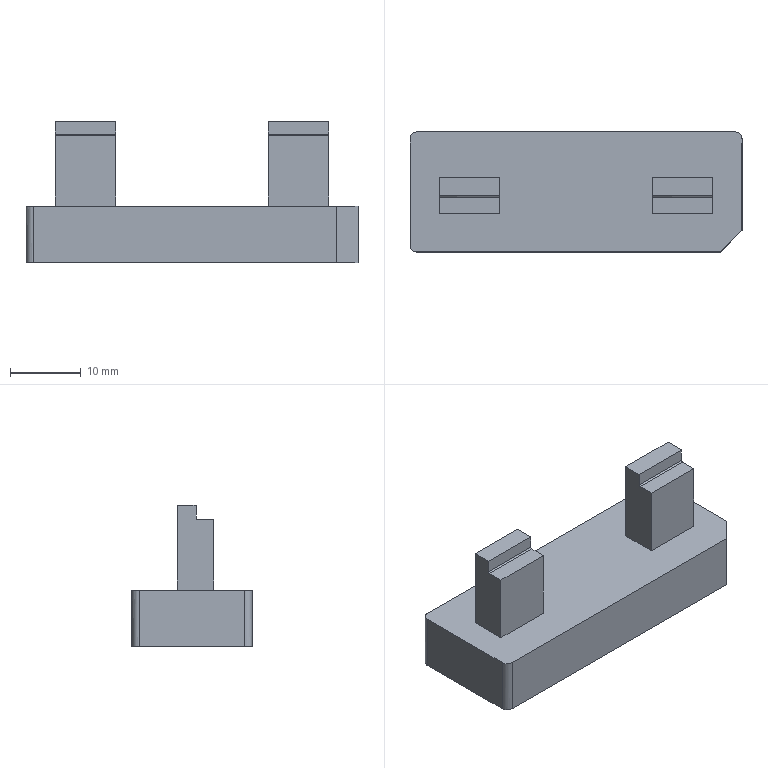NC program | PowerMill | posted by the shop | part box 47 x 17 x 19.985 mm
Lines 5811 to 7380 of 62704:
( TOOL ID   D4C_1_1 )
( TOOL DIA. 4. TIP RAD 0 LENGTH 67.16 )
( Z = -12.11 )
T2 M6
T3
G91 G28 Z0
G0 G90 G54
M08
S18000 M3
X0 Y0 M8
G43 Z9.805 H2
X-13.691 Y-3.55
Z.799
G1 Z-.401 F3600
X-13.681 Y-3.53 F6000
G3 X-13.77 Y-3.264 I-.177 J.089
G1 X-15.13 Y-2.584
X-19.278
X-19.766 Y-2.535
X-20.254 Y-2.355
X-20.509 Y-2.196
X-20.742 Y-1.995
X-20.979 Y-1.708
X-21.221 Y-1.22
X-21.319 Y-.732
X-21.322 Y2.196
X-21.23 Y2.701
X-21.008 Y3.172
X-20.742 Y3.504
X-20.567 Y3.66
X-20.254 Y3.864
X-19.766 Y4.043
X-19.278 Y4.093
X-10.981
X-10.493 Y4.065
X-10.005 Y3.917
X-9.583 Y3.66
X-9.141 Y3.172
X-9.029 Y2.973
X-8.915 Y2.684
X-8.828 Y2.196
X-8.831 Y-.732
X-8.929 Y-1.22
X-9.029 Y-1.464
X-9.171 Y-1.708
X-9.517 Y-2.097
X-9.641 Y-2.196
X-10.005 Y-2.408
X-10.493 Y-2.557
X-10.981 Y-2.584
X-15.13
X-13.691 Y-3.55 Z-.597
X-13.681 Y-3.53
G3 X-13.77 Y-3.264 I-.177 J.089
G1 X-15.13 Y-2.584
X-19.278
X-19.766 Y-2.535
X-20.254 Y-2.355
X-20.509 Y-2.196
X-20.742 Y-1.995
X-20.979 Y-1.708
X-21.221 Y-1.22
X-21.319 Y-.732
X-21.322 Y2.196
X-21.23 Y2.701
X-21.008 Y3.172
X-20.742 Y3.504
X-20.567 Y3.66
X-20.254 Y3.864
X-19.766 Y4.043
X-19.278 Y4.093
X-10.981
X-10.493 Y4.065
X-10.005 Y3.917
X-9.583 Y3.66
X-9.141 Y3.172
X-9.029 Y2.973
X-8.915 Y2.684
X-8.828 Y2.196
X-8.83 Y-.732
X-8.929 Y-1.22
X-9.029 Y-1.464
X-9.171 Y-1.708
X-9.517 Y-2.097
X-9.641 Y-2.196
X-10.005 Y-2.408
X-10.493 Y-2.557
X-10.981 Y-2.584
X-15.13
X-13.691 Y-3.55 Z-.793
X-13.681 Y-3.53
G3 X-13.77 Y-3.264 I-.177 J.089
G1 X-15.13 Y-2.584
X-19.278
X-19.766 Y-2.535
X-20.254 Y-2.355
X-20.509 Y-2.196
X-20.742 Y-1.995
X-20.979 Y-1.708
X-21.221 Y-1.22
X-21.319 Y-.732
X-21.322 Y2.196
X-21.23 Y2.701
X-21.008 Y3.172
X-20.742 Y3.504
X-20.567 Y3.66
X-20.254 Y3.864
X-19.766 Y4.043
X-19.278 Y4.093
X-10.981
X-10.493 Y4.065
X-10.005 Y3.917
X-9.583 Y3.66
X-9.141 Y3.172
X-9.029 Y2.973
X-8.915 Y2.684
X-8.828 Y2.196
X-8.83 Y-.732
X-8.929 Y-1.22
X-9.029 Y-1.464
X-9.171 Y-1.708
X-9.517 Y-2.097
X-9.641 Y-2.196
X-10.005 Y-2.409
X-10.493 Y-2.557
X-10.981 Y-2.584
X-15.13
X-13.691 Y-3.55 Z-.989
X-13.681 Y-3.53
G3 X-13.77 Y-3.264 I-.177 J.089
G1 X-15.13 Y-2.584
X-19.278
X-19.766 Y-2.535
X-20.254 Y-2.355
X-20.509 Y-2.196
X-20.742 Y-1.995
X-20.979 Y-1.708
X-21.221 Y-1.22
X-21.319 Y-.732
X-21.322 Y2.196
X-21.23 Y2.701
X-21.008 Y3.172
X-20.742 Y3.504
X-20.567 Y3.66
X-20.254 Y3.864
X-19.766 Y4.043
X-19.278 Y4.093
X-10.981
X-10.493 Y4.065
X-10.005 Y3.917
X-9.583 Y3.66
X-9.141 Y3.172
X-9.029 Y2.973
X-8.915 Y2.684
X-8.828 Y2.196
X-8.83 Y-.732
X-8.929 Y-1.22
X-9.029 Y-1.464
X-9.171 Y-1.708
X-9.517 Y-2.097
X-9.641 Y-2.196
X-10.005 Y-2.409
X-10.493 Y-2.557
X-10.981 Y-2.584
X-15.13
X-13.691 Y-3.55 Z-1.185
X-13.681 Y-3.53
G3 X-13.77 Y-3.264 I-.177 J.089
G1 X-15.13 Y-2.584
X-19.278
X-19.766 Y-2.535
X-20.254 Y-2.355
X-20.509 Y-2.196
X-20.742 Y-1.996
X-20.979 Y-1.708
X-21.221 Y-1.22
X-21.32 Y-.732
X-21.322 Y2.196
X-21.23 Y2.701
X-21.008 Y3.172
X-20.742 Y3.504
X-20.567 Y3.66
X-20.254 Y3.864
X-19.766 Y4.043
X-19.278 Y4.093
X-10.981
X-10.493 Y4.065
X-10.005 Y3.917
X-9.583 Y3.66
X-9.141 Y3.172
X-9.029 Y2.973
X-8.915 Y2.684
X-8.828 Y2.196
X-8.83 Y-.732
X-8.929 Y-1.22
X-9.029 Y-1.464
X-9.171 Y-1.708
X-9.517 Y-2.097
X-9.641 Y-2.196
X-10.005 Y-2.409
X-10.493 Y-2.557
X-10.981 Y-2.584
X-15.13
X-13.691 Y-3.55 Z-1.381
X-13.681 Y-3.53
G3 X-13.77 Y-3.264 I-.177 J.089
G1 X-15.13 Y-2.584
X-19.278
X-19.766 Y-2.535
X-20.254 Y-2.355
X-20.509 Y-2.196
X-20.742 Y-1.996
X-20.979 Y-1.708
X-21.221 Y-1.22
X-21.32 Y-.732
X-21.322 Y2.196
X-21.23 Y2.701
X-21.008 Y3.172
X-20.742 Y3.504
X-20.567 Y3.66
X-20.254 Y3.864
X-19.766 Y4.043
X-19.278 Y4.093
X-10.981
X-10.493 Y4.065
X-10.005 Y3.917
X-9.583 Y3.66
X-9.141 Y3.172
X-9.029 Y2.973
X-8.915 Y2.684
X-8.828 Y2.196
X-8.83 Y-.732
X-8.929 Y-1.22
X-9.029 Y-1.464
X-9.171 Y-1.708
X-9.517 Y-2.097
X-9.641 Y-2.196
X-10.005 Y-2.409
X-10.493 Y-2.557
X-10.981 Y-2.584
X-15.13
X-13.691 Y-3.55 Z-1.577
X-13.681 Y-3.53
G3 X-13.77 Y-3.264 I-.177 J.089
G1 X-15.13 Y-2.584
X-19.278
X-19.766 Y-2.535
X-20.254 Y-2.355
X-20.509 Y-2.196
X-20.742 Y-1.996
X-20.979 Y-1.708
X-21.221 Y-1.22
X-21.32 Y-.732
X-21.322 Y2.196
X-21.23 Y2.701
X-21.008 Y3.172
X-20.742 Y3.504
X-20.567 Y3.66
X-20.254 Y3.864
X-19.766 Y4.043
X-19.278 Y4.093
X-10.981
X-10.493 Y4.065
X-10.005 Y3.917
X-9.583 Y3.66
X-9.141 Y3.172
X-9.029 Y2.973
X-8.915 Y2.684
X-8.828 Y2.196
X-8.83 Y-.732
X-8.929 Y-1.22
X-9.029 Y-1.464
X-9.171 Y-1.708
X-9.517 Y-2.097
X-9.641 Y-2.196
X-10.005 Y-2.409
X-10.493 Y-2.557
X-10.981 Y-2.584
X-15.13
X-13.691 Y-3.55 Z-1.773
X-13.681 Y-3.53
G3 X-13.77 Y-3.264 I-.177 J.089
G1 X-15.13 Y-2.584
X-19.278
X-19.766 Y-2.535
X-20.254 Y-2.355
X-20.509 Y-2.196
X-20.742 Y-1.996
X-20.979 Y-1.708
X-21.221 Y-1.22
X-21.32 Y-.732
X-21.322 Y2.196
X-21.23 Y2.701
X-21.008 Y3.172
X-20.742 Y3.504
X-20.567 Y3.66
X-20.254 Y3.864
X-19.766 Y4.043
X-19.278 Y4.093
X-10.981
X-10.493 Y4.065
X-10.005 Y3.917
X-9.583 Y3.66
X-9.141 Y3.172
X-9.029 Y2.973
X-8.915 Y2.684
X-8.828 Y2.196
X-8.83 Y-.732
X-8.929 Y-1.22
X-9.029 Y-1.464
X-9.171 Y-1.708
X-9.517 Y-2.097
X-9.641 Y-2.196
X-10.005 Y-2.409
X-10.493 Y-2.557
X-10.981 Y-2.584
X-15.13
X-13.608 Y-3.591 Z-1.969
X-13.598 Y-3.571
G3 X-13.687 Y-3.306 I-.177 J.089
G1 X-15.13 Y-2.584
X-19.278
X-19.766 Y-2.535
X-20.254 Y-2.355
X-20.509 Y-2.196
X-20.742 Y-1.996
X-20.979 Y-1.708
X-21.221 Y-1.22
X-21.32 Y-.732
X-21.322 Y2.196
X-21.23 Y2.701
X-21.008 Y3.172
X-20.742 Y3.504
X-20.567 Y3.66
X-20.254 Y3.864
X-19.766 Y4.043
X-19.278 Y4.093
X-10.981
X-10.493 Y4.065
X-10.005 Y3.917
X-9.583 Y3.66
X-9.141 Y3.172
X-9.029 Y2.973
X-8.915 Y2.684
X-8.828 Y2.196
X-8.83 Y-.732
X-8.929 Y-1.22
X-9.029 Y-1.464
X-9.171 Y-1.708
X-9.517 Y-2.097
X-9.641 Y-2.196
X-10.005 Y-2.409
X-10.493 Y-2.557
X-10.981 Y-2.584
X-15.13
X-13.704 Y-3.64 Z-2.165
X-13.695 Y-3.62
G3 X-13.783 Y-3.354 I-.177 J.089
G1 X-15.13 Y-2.681
X-18.302
X-19.278 Y-2.686
X-19.766 Y-2.639
X-20.254 Y-2.458
X-20.636 Y-2.196
X-20.742 Y-2.097
X-21.046 Y-1.708
X-21.23 Y-1.294
X-21.324 Y-.732
X-21.322 Y2.196
X-21.23 Y2.701
X-21.008 Y3.172
X-20.742 Y3.504
X-20.567 Y3.66
X-20.254 Y3.864
X-19.766 Y4.043
X-19.278 Y4.093
X-10.981
X-10.493 Y4.065
X-10.005 Y3.917
X-9.583 Y3.66
X-9.141 Y3.172
X-9.029 Y2.973
X-8.915 Y2.684
X-8.828 Y2.196
X-8.826 Y-.732
X-8.899 Y-1.22
X-9.107 Y-1.708
X-9.517 Y-2.2
X-10.005 Y-2.506
X-10.493 Y-2.655
X-10.981 Y-2.681
X-15.13
G0 Z2.864
G1 X-13.691 Y-6.057 F10000
G0 Z-1.164
G1 Z-2.364 F3600
X-13.681 Y-6.038 F6000
G3 X-13.77 Y-5.772 I-.177 J.089
G1 X-15.13 Y-5.092
X-19.278
X-19.766 Y-5.043
X-20.254 Y-4.863
X-20.596 Y-4.637
X-20.742 Y-4.503
X-21.023 Y-4.148
X-21.23 Y-3.7
X-21.323 Y-3.172
Y-.757
Y-.745
X-21.324 Y-.732
X-21.322 Y2.105
Y2.196
X-21.23 Y2.701
X-21.008 Y3.172
X-20.742 Y3.504
X-20.567 Y3.66
X-20.254 Y3.864
X-19.766 Y4.043
X-19.278 Y4.093
X-10.981
X-10.493 Y4.065
X-10.005 Y3.917
X-9.583 Y3.66
X-9.141 Y3.172
X-9.029 Y2.973
X-8.915 Y2.684
X-8.828 Y2.196
Y2.103
X-8.826 Y-.732
X-8.827 Y-.742
Y-3.172
X-8.907 Y-3.66
X-9.029 Y-3.972
X-9.127 Y-4.148
X-9.554 Y-4.637
X-10.005 Y-4.916
X-10.493 Y-5.064
X-10.981 Y-5.092
X-15.13
X-13.691 Y-6.057 Z-2.563
X-13.681 Y-6.038
G3 X-13.77 Y-5.772 I-.177 J.089
G1 X-15.13 Y-5.092
X-19.278
X-19.766 Y-5.043
X-20.254 Y-4.863
X-20.596 Y-4.637
X-20.742 Y-4.503
X-21.023 Y-4.148
X-21.23 Y-3.7
X-21.323 Y-3.172
Y-.757
Y-.744
X-21.324 Y-.732
X-21.322 Y2.013
Y2.196
X-21.23 Y2.701
X-21.008 Y3.172
X-20.742 Y3.504
X-20.567 Y3.66
X-20.254 Y3.864
X-19.766 Y4.043
X-19.278 Y4.093
X-10.981
X-10.493 Y4.065
X-10.005 Y3.917
X-9.583 Y3.66
X-9.141 Y3.172
X-9.029 Y2.973
X-8.915 Y2.684
X-8.828 Y2.196
Y2.008
X-8.826 Y-.732
X-8.827 Y-.742
Y-3.172
X-8.907 Y-3.66
X-9.029 Y-3.972
X-9.127 Y-4.148
X-9.554 Y-4.637
X-10.005 Y-4.916
X-10.493 Y-5.064
X-10.981 Y-5.092
X-15.13
X-13.691 Y-6.057 Z-2.762
X-13.681 Y-6.038
G3 X-13.77 Y-5.772 I-.177 J.089
G1 X-15.13 Y-5.092
X-19.278
X-19.766 Y-5.043
X-20.254 Y-4.863
X-20.596 Y-4.637
X-20.742 Y-4.503
X-21.023 Y-4.148
X-21.23 Y-3.7
X-21.323 Y-3.172
Y-.756
Y-.744
X-21.324 Y-.732
X-21.322 Y1.922
Y2.196
X-21.23 Y2.701
X-21.009 Y3.172
X-20.742 Y3.504
X-20.567 Y3.66
X-20.254 Y3.864
X-19.766 Y4.043
X-19.278 Y4.093
X-10.981
X-10.493 Y4.065
X-10.005 Y3.917
X-9.583 Y3.66
X-9.141 Y3.172
X-9.029 Y2.973
X-8.915 Y2.684
X-8.828 Y2.196
Y1.913
X-8.826 Y-.732
X-8.827 Y-.742
Y-3.172
X-8.907 Y-3.66
X-9.029 Y-3.972
X-9.127 Y-4.148
X-9.554 Y-4.637
X-10.005 Y-4.916
X-10.493 Y-5.064
X-10.981 Y-5.092
X-15.13
X-13.691 Y-6.057 Z-2.961
X-13.681 Y-6.038
G3 X-13.77 Y-5.772 I-.177 J.089
G1 X-15.13 Y-5.092
X-19.278
X-19.766 Y-5.043
X-20.254 Y-4.863
X-20.596 Y-4.637
X-20.742 Y-4.503
X-21.023 Y-4.148
X-21.23 Y-3.7
X-21.323 Y-3.172
Y-.756
Y-.744
X-21.324 Y-.732
X-21.322 Y1.83
Y2.196
X-21.23 Y2.701
X-21.009 Y3.172
X-20.742 Y3.504
X-20.567 Y3.66
X-20.254 Y3.864
X-19.766 Y4.043
X-19.278 Y4.093
X-10.981
X-10.493 Y4.065
X-10.005 Y3.917
X-9.583 Y3.66
X-9.141 Y3.172
X-9.029 Y2.973
X-8.915 Y2.684
X-8.828 Y2.196
Y1.818
X-8.826 Y-.732
X-8.827 Y-.741
Y-3.172
X-8.907 Y-3.66
X-9.029 Y-3.972
X-9.127 Y-4.148
X-9.554 Y-4.637
X-10.005 Y-4.916
X-10.493 Y-5.064
X-10.981 Y-5.092
X-15.13
X-13.691 Y-6.057 Z-3.16
X-13.681 Y-6.038
G3 X-13.77 Y-5.772 I-.177 J.089
G1 X-15.13 Y-5.092
X-19.278
X-19.766 Y-5.043
X-20.254 Y-4.863
X-20.596 Y-4.637
X-20.742 Y-4.503
X-21.023 Y-4.148
X-21.23 Y-3.7
X-21.323 Y-3.172
Y-.756
Y-.744
X-21.324 Y-.732
X-21.322 Y1.738
Y2.196
X-21.23 Y2.701
X-21.009 Y3.172
X-20.742 Y3.504
X-20.567 Y3.66
X-20.254 Y3.864
X-19.766 Y4.043
X-19.278 Y4.093
X-10.981
X-10.493 Y4.065
X-10.005 Y3.917
X-9.583 Y3.66
X-9.141 Y3.172
X-9.029 Y2.973
X-8.915 Y2.684
X-8.828 Y2.196
Y1.723
X-8.826 Y-.732
X-8.827 Y-.741
Y-3.172
X-8.907 Y-3.66
X-9.029 Y-3.972
X-9.127 Y-4.148
X-9.554 Y-4.637
X-10.005 Y-4.916
X-10.493 Y-5.064
X-10.981 Y-5.092
X-15.13
X-13.691 Y-6.057 Z-3.358
X-13.681 Y-6.038
G3 X-13.77 Y-5.772 I-.177 J.089
G1 X-15.13 Y-5.092
X-19.278
X-19.766 Y-5.043
X-20.254 Y-4.863
X-20.596 Y-4.637
X-20.742 Y-4.503
X-21.023 Y-4.148
X-21.23 Y-3.7
X-21.323 Y-3.172
Y-.755
Y-.744
X-21.324 Y-.732
X-21.322 Y1.647
Y2.196
X-21.23 Y2.701
X-21.009 Y3.172
X-20.742 Y3.504
X-20.567 Y3.66
X-20.254 Y3.864
X-19.766 Y4.043
X-19.278 Y4.093
X-10.981
X-10.493 Y4.065
X-10.005 Y3.917
X-9.583 Y3.66
X-9.141 Y3.172
X-9.029 Y2.973
X-8.915 Y2.684
X-8.828 Y2.196
Y1.628
X-8.826 Y-.732
X-8.827 Y-.741
Y-3.172
X-8.907 Y-3.66
X-9.029 Y-3.972
X-9.127 Y-4.148
X-9.554 Y-4.637
X-10.005 Y-4.916
X-10.493 Y-5.064
X-10.981 Y-5.092
X-15.13
X-13.691 Y-6.057 Z-3.557
X-13.681 Y-6.038
G3 X-13.77 Y-5.772 I-.177 J.089
G1 X-15.13 Y-5.092
X-19.278
X-19.766 Y-5.043
X-20.254 Y-4.863
X-20.596 Y-4.637
X-20.742 Y-4.503
X-21.023 Y-4.148
X-21.23 Y-3.7
X-21.323 Y-3.172
Y-.755
Y-.743
X-21.324 Y-.732
X-21.322 Y1.555
Y2.196
X-21.23 Y2.701
X-21.009 Y3.172
X-20.742 Y3.504
X-20.567 Y3.66
X-20.254 Y3.864
X-19.766 Y4.043
X-19.278 Y4.093
X-10.981
X-10.493 Y4.065
X-10.005 Y3.917
X-9.583 Y3.66
X-9.141 Y3.172
X-9.029 Y2.973
X-8.914 Y2.684
X-8.828 Y2.196
Y1.533
X-8.826 Y-.732
X-8.827 Y-.74
Y-3.172
X-8.907 Y-3.66
X-9.029 Y-3.972
X-9.127 Y-4.148
X-9.554 Y-4.637
X-10.005 Y-4.916
X-10.493 Y-5.064
X-10.981 Y-5.092
X-15.13
X-13.691 Y-6.057 Z-3.756
X-13.681 Y-6.038
G3 X-13.77 Y-5.772 I-.177 J.089
G1 X-15.13 Y-5.092
X-19.278
X-19.766 Y-5.043
X-20.254 Y-4.863
X-20.596 Y-4.637
X-20.742 Y-4.503
X-21.023 Y-4.148
X-21.23 Y-3.7
X-21.323 Y-3.172
Y-.754
Y-.743
X-21.324 Y-.732
X-21.322 Y1.464
Y2.196
X-21.23 Y2.701
X-21.009 Y3.172
X-20.742 Y3.504
X-20.567 Y3.66
X-20.254 Y3.864
X-19.766 Y4.043
X-19.278 Y4.093
X-10.981
X-10.493 Y4.065
X-10.005 Y3.917
X-9.583 Y3.66
X-9.141 Y3.172
X-9.029 Y2.973
X-8.914 Y2.684
X-8.828 Y2.196
Y1.438
X-8.826 Y-.732
X-8.827 Y-.74
Y-3.172
X-8.907 Y-3.66
X-9.029 Y-3.972
X-9.127 Y-4.148
X-9.554 Y-4.637
X-10.005 Y-4.916
X-10.493 Y-5.064
X-10.981 Y-5.092
X-15.13
X-13.691 Y-6.057 Z-3.955
X-13.681 Y-6.038
G3 X-13.77 Y-5.772 I-.177 J.089
G1 X-15.13 Y-5.092
X-19.278
X-19.766 Y-5.043
X-20.254 Y-4.863
X-20.596 Y-4.637
X-20.742 Y-4.503
X-21.023 Y-4.148
X-21.23 Y-3.7
X-21.323 Y-3.172
Y-.754
Y-.743
X-21.324 Y-.732
X-21.322 Y1.372
Y2.196
X-21.23 Y2.701
X-21.009 Y3.172
X-20.742 Y3.504
X-20.567 Y3.66
X-20.254 Y3.864
X-19.766 Y4.043
X-19.278 Y4.093
X-10.981
X-10.493 Y4.065
X-10.005 Y3.917
X-9.583 Y3.66
X-9.141 Y3.172
X-9.029 Y2.973
X-8.914 Y2.684
X-8.828 Y2.196
Y1.344
X-8.826 Y-.732
X-8.827 Y-.74
Y-3.172
X-8.907 Y-3.66
X-9.029 Y-3.972
X-9.127 Y-4.148
X-9.554 Y-4.637
X-10.005 Y-4.916
X-10.493 Y-5.064
X-10.981 Y-5.092
X-15.13
X-13.691 Y-6.057 Z-4.154
X-13.681 Y-6.038
G3 X-13.77 Y-5.772 I-.177 J.089
G1 X-15.13 Y-5.092
X-19.278
X-19.766 Y-5.043
X-20.254 Y-4.863
X-20.596 Y-4.637
X-20.742 Y-4.503
X-21.023 Y-4.148
X-21.23 Y-3.7
X-21.323 Y-3.172
Y-.753
Y-.743
X-21.324 Y-.732
X-21.322 Y1.28
Y2.196
X-21.23 Y2.701
X-21.009 Y3.172
X-20.742 Y3.504
X-20.567 Y3.66
X-20.254 Y3.864
X-19.766 Y4.043
X-19.278 Y4.093
X-10.981
X-10.493 Y4.065
X-10.005 Y3.917
X-9.583 Y3.66
X-9.141 Y3.172
X-9.029 Y2.973
X-8.914 Y2.684
X-8.828 Y2.196
X-8.827 Y1.249
X-8.826 Y-.732
X-8.827 Y-.739
Y-3.172
X-8.907 Y-3.66
X-9.029 Y-3.972
X-9.127 Y-4.148
X-9.554 Y-4.637
X-10.005 Y-4.916
X-10.493 Y-5.064
X-10.981 Y-5.092
X-15.13
X-13.691 Y-6.057 Z-4.353
X-13.681 Y-6.038
G3 X-13.77 Y-5.772 I-.177 J.089
G1 X-15.13 Y-5.092
X-19.278
X-19.766 Y-5.043
X-20.254 Y-4.863
X-20.596 Y-4.637
X-20.742 Y-4.503
X-21.023 Y-4.148
X-21.23 Y-3.7
X-21.323 Y-3.172
Y-.753
Y-.742
X-21.324 Y-.732
X-21.322 Y1.189
Y2.196
X-21.23 Y2.701
X-21.009 Y3.172
X-20.742 Y3.504
X-20.567 Y3.66
X-20.254 Y3.864
X-19.766 Y4.043
X-19.278 Y4.093
X-10.981
X-10.493 Y4.065
X-10.005 Y3.917
X-9.583 Y3.66
X-9.141 Y3.172
X-9.029 Y2.973
X-8.914 Y2.684
X-8.828 Y2.196
X-8.827 Y1.154
X-8.826 Y-.732
X-8.827 Y-.739
Y-3.172
X-8.907 Y-3.66
X-9.029 Y-3.972
X-9.127 Y-4.148
X-9.554 Y-4.637
X-10.005 Y-4.916
X-10.493 Y-5.064
X-10.981 Y-5.092
X-15.13
X-13.691 Y-6.057 Z-4.552
X-13.681 Y-6.038
G3 X-13.77 Y-5.772 I-.177 J.089
G1 X-15.13 Y-5.092
X-19.278
X-19.766 Y-5.043
X-20.254 Y-4.863
X-20.596 Y-4.637
X-20.742 Y-4.503
X-21.023 Y-4.148
X-21.23 Y-3.7
X-21.323 Y-3.172
Y-.752
Y-.742
X-21.324 Y-.732
X-21.322 Y1.097
Y2.196
X-21.23 Y2.701
X-21.009 Y3.172
X-20.742 Y3.504
X-20.567 Y3.66
X-20.254 Y3.864
X-19.766 Y4.043
X-19.278 Y4.093
X-10.981
X-10.493 Y4.065
X-10.005 Y3.917
X-9.583 Y3.66
X-9.141 Y3.172
X-9.029 Y2.973
X-8.914 Y2.684
X-8.828 Y2.196
X-8.827 Y1.059
X-8.826 Y-.732
X-8.827 Y-.739
Y-3.172
X-8.907 Y-3.66
X-9.029 Y-3.972
X-9.127 Y-4.148
X-9.554 Y-4.637
X-10.005 Y-4.916
X-10.493 Y-5.064
X-10.981 Y-5.092
X-15.13
X-13.691 Y-6.057 Z-4.751
X-13.681 Y-6.038
G3 X-13.77 Y-5.772 I-.177 J.089
G1 X-15.13 Y-5.092
X-19.278
X-19.766 Y-5.043
X-20.254 Y-4.863
X-20.596 Y-4.637
X-20.742 Y-4.503
X-21.023 Y-4.148
X-21.23 Y-3.7
X-21.323 Y-3.172
Y-.752
Y-.742
X-21.324 Y-.732
X-21.323 Y1.005
X-21.322 Y2.196
X-21.23 Y2.701
X-21.009 Y3.172
X-20.742 Y3.504
X-20.567 Y3.66
X-20.254 Y3.864
X-19.766 Y4.043
X-19.278 Y4.093
X-10.981
X-10.493 Y4.065
X-10.005 Y3.917
X-9.583 Y3.66
X-9.141 Y3.172
X-9.029 Y2.973
X-8.914 Y2.684
X-8.828 Y2.196
X-8.827 Y.964
X-8.826 Y-.732
X-8.827 Y-.738
Y-3.172
X-8.907 Y-3.66
X-9.029 Y-3.972
X-9.127 Y-4.148
X-9.554 Y-4.637
X-10.005 Y-4.916
X-10.493 Y-5.064
X-10.981 Y-5.092
X-15.13
X-13.691 Y-6.057 Z-4.95
X-13.681 Y-6.038
G3 X-13.77 Y-5.772 I-.177 J.089
G1 X-15.13 Y-5.092
X-19.278
X-19.766 Y-5.043
X-20.254 Y-4.863
X-20.596 Y-4.637
X-20.742 Y-4.503
X-21.023 Y-4.148
X-21.23 Y-3.7
X-21.323 Y-3.172
Y-.751
Y-.742
X-21.324 Y-.732
X-21.323 Y.913
X-21.322 Y2.196
X-21.23 Y2.701
X-21.009 Y3.172
X-20.742 Y3.504
X-20.567 Y3.66
X-20.254 Y3.864
X-19.766 Y4.043
X-19.278 Y4.093
X-10.981
X-10.493 Y4.065
X-10.005 Y3.917
X-9.583 Y3.66
X-9.141 Y3.172
X-9.029 Y2.973
X-8.914 Y2.684
X-8.828 Y2.196
X-8.827 Y.868
X-8.826 Y-.732
X-8.827 Y-.738
Y-3.172
X-8.907 Y-3.66
X-9.029 Y-3.972
X-9.127 Y-4.148
X-9.554 Y-4.637
X-10.005 Y-4.916
X-10.493 Y-5.064
X-10.981 Y-5.092
X-15.13
X-13.691 Y-6.057 Z-5.149
X-13.681 Y-6.038
G3 X-13.77 Y-5.772 I-.177 J.089
G1 X-15.13 Y-5.092
X-19.278
X-19.766 Y-5.043
X-20.254 Y-4.863
X-20.596 Y-4.637
X-20.742 Y-4.503
X-21.023 Y-4.148
X-21.23 Y-3.7
X-21.323 Y-3.172
Y-.751
Y-.741
X-21.324 Y-.732
X-21.323 Y.822
X-21.322 Y2.196
X-21.23 Y2.701
X-21.009 Y3.172
X-20.742 Y3.504
X-20.567 Y3.66
X-20.254 Y3.864
X-19.766 Y4.043
X-19.278 Y4.093
X-10.981
X-10.493 Y4.065
X-10.005 Y3.917
X-9.583 Y3.66
X-9.141 Y3.172
X-9.029 Y2.973
X-8.914 Y2.684
X-8.828 Y2.196
X-8.827 Y.773
X-8.826 Y-.732
X-8.827 Y-.738
Y-3.172
X-8.907 Y-3.66
X-9.029 Y-3.972
X-9.127 Y-4.148
X-9.554 Y-4.637
X-10.005 Y-4.916
X-10.493 Y-5.064
X-10.981 Y-5.092
X-15.13
X-13.691 Y-6.057 Z-5.347
X-13.681 Y-6.038
G3 X-13.77 Y-5.772 I-.177 J.089
G1 X-15.13 Y-5.092
X-19.278
X-19.766 Y-5.043
X-20.254 Y-4.863
X-20.596 Y-4.637
X-20.742 Y-4.503
X-21.023 Y-4.148
X-21.23 Y-3.7
X-21.323 Y-3.172
Y-.75
Y-.741
X-21.324 Y-.732
X-21.323 Y.73
X-21.322 Y2.196
X-21.23 Y2.701
X-21.009 Y3.172
X-20.742 Y3.504
X-20.567 Y3.66
X-20.254 Y3.864
X-19.766 Y4.043
X-19.278 Y4.093
X-10.981
X-10.493 Y4.065
X-10.005 Y3.917
X-9.583 Y3.66
X-9.141 Y3.172
X-9.029 Y2.973
X-8.914 Y2.684
X-8.828 Y2.196
X-8.827 Y.678
X-8.826 Y-.732
X-8.827 Y-.737
Y-3.172
X-8.907 Y-3.66
X-9.029 Y-3.972
X-9.127 Y-4.148
X-9.554 Y-4.637
X-10.005 Y-4.916
X-10.493 Y-5.064
X-10.981 Y-5.092
X-15.13
X-13.691 Y-6.057 Z-5.546
X-13.681 Y-6.038
G3 X-13.77 Y-5.772 I-.177 J.089
G1 X-15.13 Y-5.092
X-19.278
X-19.766 Y-5.043
X-20.254 Y-4.863
X-20.596 Y-4.637
X-20.742 Y-4.503
X-21.023 Y-4.148
X-21.23 Y-3.7
X-21.323 Y-3.172
Y-.749
Y-.741
X-21.324 Y-.732
X-21.323 Y.641
X-21.322 Y2.196
X-21.23 Y2.701
X-21.009 Y3.172
X-20.742 Y3.504
X-20.567 Y3.66
X-20.254 Y3.864
X-19.766 Y4.043
X-19.278 Y4.093
X-10.981
X-10.493 Y4.065
X-10.005 Y3.917
X-9.583 Y3.66
X-9.141 Y3.172
X-9.029 Y2.973
X-8.914 Y2.684
X-8.828 Y2.196
X-8.827 Y.584
X-8.826 Y-.732
X-8.827 Y-.737
Y-3.172
X-8.907 Y-3.66
X-9.029 Y-3.972
X-9.127 Y-4.148
X-9.554 Y-4.637
X-10.005 Y-4.916
X-10.493 Y-5.064
X-10.981 Y-5.092
X-15.13
X-13.691 Y-6.057 Z-5.745
X-13.681 Y-6.038
G3 X-13.77 Y-5.772 I-.177 J.089
G1 X-15.13 Y-5.092
X-19.278
X-19.766 Y-5.043
X-20.254 Y-4.863
X-20.596 Y-4.637
X-20.742 Y-4.503
X-21.023 Y-4.148
X-21.23 Y-3.7
X-21.323 Y-3.172
Y-.749
Y-.74
X-21.324 Y-.732
X-21.323 Y.549
X-21.322 Y2.196
X-21.23 Y2.701
X-21.009 Y3.172
X-20.742 Y3.504
X-20.567 Y3.66
X-20.254 Y3.864
X-19.766 Y4.043
X-19.278 Y4.093
X-10.981
X-10.493 Y4.065
X-10.005 Y3.917
X-9.583 Y3.66
X-9.141 Y3.172
X-9.029 Y2.973
X-8.914 Y2.684
X-8.828 Y2.196
X-8.827 Y.489
X-8.826 Y-.732
X-8.827 Y-.736
Y-3.172
X-8.907 Y-3.66
X-9.029 Y-3.972
X-9.127 Y-4.148
X-9.554 Y-4.637
X-10.005 Y-4.916
X-10.493 Y-5.064
X-10.981 Y-5.092
X-15.13
X-13.691 Y-6.057 Z-5.944
X-13.681 Y-6.038
G3 X-13.77 Y-5.772 I-.177 J.089
G1 X-15.13 Y-5.092
X-19.278
X-19.766 Y-5.043
X-20.254 Y-4.863
X-20.596 Y-4.637
X-20.742 Y-4.503
X-21.023 Y-4.148
X-21.23 Y-3.7
X-21.323 Y-3.172
Y-.748
Y-.74
X-21.324 Y-.732
X-21.323 Y.457
X-21.322 Y2.196
X-21.23 Y2.701
X-21.009 Y3.172
X-20.742 Y3.504
X-20.567 Y3.66
X-20.254 Y3.864
X-19.766 Y4.043
X-19.278 Y4.093
X-10.981
X-10.493 Y4.065
X-10.005 Y3.917
X-9.583 Y3.66
X-9.141 Y3.172
X-9.029 Y2.973
X-8.914 Y2.684
X-8.828 Y2.196
X-8.827 Y.394
X-8.826 Y-.732
X-8.827 Y-.736
Y-3.172
X-8.907 Y-3.66
X-9.029 Y-3.972
X-9.127 Y-4.148
X-9.554 Y-4.637
X-10.005 Y-4.916
X-10.493 Y-5.064
X-10.981 Y-5.092
X-15.13
X-13.691 Y-6.057 Z-6.143
X-13.681 Y-6.038
G3 X-13.77 Y-5.772 I-.177 J.089
G1 X-15.13 Y-5.092
X-19.278
X-19.766 Y-5.043
X-20.254 Y-4.863
X-20.596 Y-4.637
X-20.742 Y-4.503
X-21.023 Y-4.148
X-21.23 Y-3.7
X-21.323 Y-3.172
Y-.748
Y-.74
Y-.732
Y.364
X-21.322 Y2.196
X-21.23 Y2.701
X-21.009 Y3.172
X-20.742 Y3.504
X-20.567 Y3.66
X-20.254 Y3.864
X-19.766 Y4.043
X-19.278 Y4.093
X-10.981
X-10.493 Y4.065
X-10.005 Y3.917
X-9.583 Y3.66
X-9.141 Y3.172
X-9.029 Y2.973
X-8.914 Y2.684
X-8.828 Y2.196
X-8.827 Y.298
Y-.732
Y-.736
Y-3.172
X-8.907 Y-3.66
X-9.029 Y-3.972
X-9.127 Y-4.148
X-9.554 Y-4.637
X-10.005 Y-4.916
X-10.493 Y-5.064
X-10.981 Y-5.092
X-15.13
X-13.691 Y-6.057 Z-6.342
X-13.681 Y-6.038
G3 X-13.77 Y-5.772 I-.177 J.089
G1 X-15.13 Y-5.092
X-19.278
X-19.766 Y-5.043
X-20.254 Y-4.863
X-20.596 Y-4.637
X-20.742 Y-4.503
X-21.023 Y-4.148
X-21.23 Y-3.7
X-21.323 Y-3.172
Y-.747
Y-.739
Y-.732
Y.273
X-21.322 Y2.196
X-21.23 Y2.701
X-21.009 Y3.172
X-20.742 Y3.504
X-20.567 Y3.66
X-20.254 Y3.864
X-19.766 Y4.043
X-19.278 Y4.093
X-10.981
X-10.493 Y4.065
X-10.005 Y3.917
X-9.583 Y3.66
X-9.141 Y3.172
X-9.029 Y2.973
X-8.914 Y2.684
X-8.828 Y2.196
X-8.827 Y.203
Y-.732
Y-.735
Y-3.172
X-8.907 Y-3.66
X-9.029 Y-3.972
X-9.127 Y-4.148
X-9.554 Y-4.637
X-10.005 Y-4.916
X-10.493 Y-5.064
X-10.981 Y-5.092
X-15.13
X-13.691 Y-6.057 Z-6.541
X-13.681 Y-6.038
G3 X-13.77 Y-5.772 I-.177 J.089
G1 X-15.13 Y-5.092
X-19.278
X-19.766 Y-5.043
X-20.254 Y-4.863
X-20.596 Y-4.637
X-20.742 Y-4.503
X-21.023 Y-4.148
X-21.23 Y-3.7
X-21.323 Y-3.172
Y-.746
Y-.739
Y-.732
Y.181
X-21.322 Y2.196
X-21.23 Y2.701
X-21.009 Y3.172
X-20.742 Y3.504
X-20.567 Y3.66
X-20.254 Y3.864
X-19.766 Y4.043
X-19.278 Y4.093
X-10.981
X-10.493 Y4.065
X-10.005 Y3.917
X-9.583 Y3.66
X-9.141 Y3.172
X-9.029 Y2.973
X-8.914 Y2.684
X-8.828 Y2.196
X-8.827 Y.107
Y-.732
Y-.735
Y-3.172
X-8.907 Y-3.66
X-9.029 Y-3.972
X-9.127 Y-4.148
X-9.554 Y-4.637
X-10.005 Y-4.916
X-10.493 Y-5.064
X-10.981 Y-5.092
X-15.13
X-13.691 Y-6.057 Z-6.74
X-13.681 Y-6.038
G3 X-13.77 Y-5.772 I-.177 J.089
G1 X-15.13 Y-5.092
X-19.278
X-19.766 Y-5.043
X-20.254 Y-4.863
X-20.596 Y-4.637
X-20.742 Y-4.503
X-21.023 Y-4.148
X-21.23 Y-3.7
X-21.323 Y-3.172
Y-.746
Y-.739
Y-.732
Y.089
X-21.322 Y2.196
X-21.23 Y2.701
X-21.009 Y3.172
X-20.742 Y3.504
X-20.567 Y3.66
X-20.254 Y3.864
X-19.766 Y4.043
X-19.278 Y4.093
X-10.981
X-10.493 Y4.065
X-10.005 Y3.917
X-9.583 Y3.66
X-9.141 Y3.172
X-9.029 Y2.973
X-8.914 Y2.684
X-8.828 Y2.196
X-8.827 Y.012
Y-.732
Y-.735
Y-3.172
X-8.907 Y-3.66
X-9.029 Y-3.972
X-9.127 Y-4.148
X-9.554 Y-4.637
X-10.005 Y-4.916
X-10.493 Y-5.064
X-10.981 Y-5.092
X-15.13
X-13.691 Y-6.057 Z-6.939
X-13.681 Y-6.038
G3 X-13.77 Y-5.772 I-.177 J.089
G1 X-15.13 Y-5.092
X-19.278
X-19.766 Y-5.043
X-20.254 Y-4.863
X-20.596 Y-4.637
X-20.742 Y-4.503
X-21.023 Y-4.148
X-21.23 Y-3.7
X-21.323 Y-3.172
Y-.745
Y-.738
Y-.732
Y-.003
X-21.322 Y2.196
X-21.23 Y2.701
X-21.009 Y3.172
X-20.742 Y3.504
X-20.567 Y3.66
X-20.254 Y3.864
X-19.766 Y4.043
X-19.278 Y4.093
X-10.981
X-10.493 Y4.065
X-10.005 Y3.917
X-9.583 Y3.66
X-9.141 Y3.172
X-9.029 Y2.973
X-8.914 Y2.684
X-8.828 Y2.196
X-8.827 Y-.084
Y-.732
Y-.734
Y-3.172
X-8.907 Y-3.66
X-9.029 Y-3.972
X-9.127 Y-4.148
X-9.554 Y-4.637
X-10.005 Y-4.916
X-10.493 Y-5.064
X-10.981 Y-5.092
X-15.13
X-13.691 Y-6.057 Z-7.138
X-13.681 Y-6.038
G3 X-13.77 Y-5.772 I-.177 J.089
G1 X-15.13 Y-5.092
X-19.278
X-19.766 Y-5.043
X-20.254 Y-4.863
X-20.596 Y-4.637
X-20.742 Y-4.503
X-21.023 Y-4.148
X-21.23 Y-3.7
X-21.323 Y-3.172
Y-.744
Y-.738
Y-.732
Y-.094
X-21.322 Y2.196
X-21.23 Y2.701
X-21.009 Y3.172
X-20.742 Y3.504
X-20.567 Y3.66
X-20.254 Y3.864
X-19.766 Y4.043
X-19.278 Y4.093
X-10.981
X-10.493 Y4.065
X-10.005 Y3.917
X-9.583 Y3.66
X-9.141 Y3.172
X-9.029 Y2.973
X-8.914 Y2.684
X-8.828 Y2.196
X-8.827 Y-.179
Y-.732
Y-.734
Y-3.172
X-8.907 Y-3.66
X-9.029 Y-3.972
X-9.127 Y-4.148
X-9.554 Y-4.637
X-10.005 Y-4.916
X-10.493 Y-5.064
X-10.981 Y-5.092
X-15.13
X-13.691 Y-6.057 Z-7.336
X-13.681 Y-6.038
G3 X-13.77 Y-5.772 I-.177 J.089
G1 X-15.13 Y-5.092
X-19.278
X-19.766 Y-5.043
X-20.254 Y-4.863
X-20.596 Y-4.637
X-20.742 Y-4.503
X-21.023 Y-4.148
X-21.23 Y-3.7
X-21.323 Y-3.172
Y-.743
Y-.737
Y-.732
Y-.186
X-21.322 Y2.196
X-21.23 Y2.701
X-21.009 Y3.172
X-20.742 Y3.504
X-20.567 Y3.66
X-20.254 Y3.864
X-19.766 Y4.043
X-19.278 Y4.093
X-10.981
X-10.493 Y4.065
X-10.005 Y3.917
X-9.583 Y3.66
X-9.141 Y3.172
X-9.029 Y2.973
X-8.914 Y2.684
X-8.828 Y2.196
X-8.827 Y-.273
Y-.732
Y-.734
Y-3.172
X-8.907 Y-3.66
X-9.029 Y-3.972
X-9.127 Y-4.148
X-9.554 Y-4.637
X-10.005 Y-4.916
X-10.493 Y-5.064
X-10.981 Y-5.092
X-15.13
X-13.691 Y-6.057 Z-7.535
X-13.681 Y-6.038
G3 X-13.77 Y-5.772 I-.177 J.089
G1 X-15.13 Y-5.092
X-19.278
X-19.766 Y-5.043
X-20.254 Y-4.863
X-20.596 Y-4.637
X-20.742 Y-4.503
X-21.023 Y-4.148
X-21.23 Y-3.7
X-21.323 Y-3.172
Y-.742
Y-.737
Y-.732
Y-.28
X-21.322 Y2.196
X-21.23 Y2.701
X-21.009 Y3.172
X-20.742 Y3.504
X-20.567 Y3.66
X-20.254 Y3.864
X-19.766 Y4.043
X-19.278 Y4.093
X-10.981
X-10.493 Y4.065
X-10.005 Y3.917
X-9.583 Y3.66
X-9.141 Y3.172
X-9.029 Y2.973
X-8.914 Y2.684